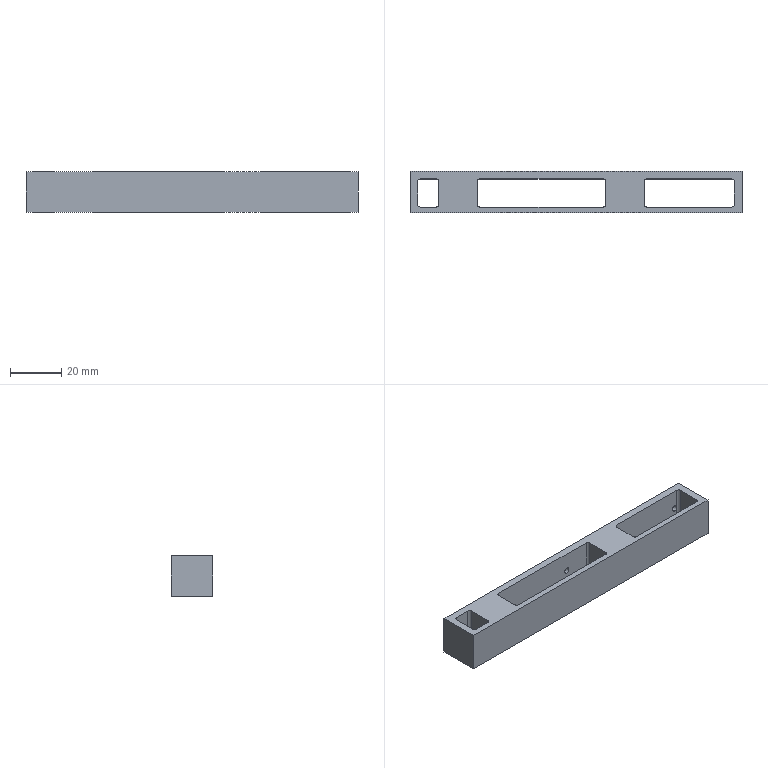NC program | NX | posted with a generic post | part box 130 x 16.2 x 16 mm
Lines 949 to 1955 of 19599:
(ZLEVEL_PROFILE_COPY_1_COPY , TOOL : D2)
N1872 T02 M6
N1874 G54
N1876 G17 G0 G90 X-57.176 Y-4.3 B0. C0. S9500 M3
N1878 G43 Z30. H2
N1880 Z0.401
N1882 G94 G1 Z-0.099 F1000.
N1884 X-56.888 Y-4.8
N1886 G3 X-56.715 Y-4.9 R0.2
N1888 G1 X-54.708 F2000.
N1890 Y-2.894
N1892 G3 X-54.808 Y-2.72 R0.2
N1894 G1 X-55.308 Y-2.432
N1896 Z0.401
N1898 G0 X-57.176 Y-4.3 Z0.301
N1900 G1 Z-0.199 F1000.
N1902 X-56.888 Y-4.8
N1904 G3 X-56.715 Y-4.9 R0.2
N1906 G1 X-54.708 F2000.
N1908 Y-2.894
N1910 G3 X-54.808 Y-2.72 R0.2
N1912 G1 X-55.308 Y-2.432
N1914 Z0.301
N1916 G0 X-57.176 Y-4.3 Z0.202
N1918 G1 Z-0.298 F1000.
N1920 X-56.888 Y-4.8
N1922 G3 X-56.715 Y-4.9 R0.2
N1924 G1 X-54.708 F2000.
N1926 Y-2.894
N1928 G3 X-54.808 Y-2.72 R0.2
N1930 G1 X-55.308 Y-2.432
N1932 Z0.202
N1934 G0 X-57.176 Y-4.3 Z0.102
N1936 G1 Z-0.398 F1000.
N1938 X-56.888 Y-4.8
N1940 G3 X-56.715 Y-4.9 R0.2
N1942 G1 X-54.708 F2000.
N1944 Y-2.894
N1946 G3 X-54.808 Y-2.72 R0.2
N1948 G1 X-55.308 Y-2.432
N1950 Z0.102
N1952 G0 X-57.176 Y-4.3 Z0.003
N1954 G1 Z-0.497 F1000.
N1956 X-56.888 Y-4.8
N1958 G3 X-56.715 Y-4.9 R0.2
N1960 G1 X-54.708 F2000.
N1962 Y-2.894
N1964 G3 X-54.808 Y-2.72 R0.2
N1966 G1 X-55.308 Y-2.432
N1968 Z0.003
N1970 G0 X-57.176 Y-4.3 Z-0.096
N1972 G1 Z-0.596 F1000.
N1974 X-56.888 Y-4.8
N1976 G3 X-56.715 Y-4.9 R0.2
N1978 G1 X-54.708 F2000.
N1980 Y-2.894
N1982 G3 X-54.808 Y-2.72 R0.2
N1984 G1 X-55.308 Y-2.432
N1986 Z-0.096
N1988 G0 X-57.176 Y-4.3 Z-0.196
N1990 G1 Z-0.696 F1000.
N1992 X-56.888 Y-4.8
N1994 G3 X-56.715 Y-4.9 R0.2
N1996 G1 X-54.708 F2000.
N1998 Y-2.894
N2000 G3 X-54.808 Y-2.72 R0.2
N2002 G1 X-55.308 Y-2.432
N2004 Z-0.196
N2006 G0 X-57.176 Y-4.3 Z-0.295
N2008 G1 Z-0.795 F1000.
N2010 X-56.888 Y-4.8
N2012 G3 X-56.715 Y-4.9 R0.2
N2014 G1 X-54.708 F2000.
N2016 Y-2.894
N2018 G3 X-54.808 Y-2.72 R0.2
N2020 G1 X-55.308 Y-2.432
N2022 Z-0.295
N2024 G0 X-57.176 Y-4.3 Z-0.394
N2026 G1 Z-0.894 F1000.
N2028 X-56.888 Y-4.8
N2030 G3 X-56.715 Y-4.9 R0.2
N2032 G1 X-54.708 F2000.
N2034 Y-2.894
N2036 G3 X-54.808 Y-2.72 R0.2
N2038 G1 X-55.308 Y-2.432
N2040 Z-0.394
N2042 G0 X-57.176 Y-4.3 Z-0.494
N2044 G1 Z-0.994 F1000.
N2046 X-56.888 Y-4.8
N2048 G3 X-56.715 Y-4.9 R0.2
N2050 G1 X-54.708 F2000.
N2052 Y-2.894
N2054 G3 X-54.808 Y-2.72 R0.2
N2056 G1 X-55.308 Y-2.432
N2058 Z-0.494
N2060 G0 X-57.176 Y-4.3 Z-0.593
N2062 G1 Z-1.093 F1000.
N2064 X-56.888 Y-4.8
N2066 G3 X-56.715 Y-4.9 R0.2
N2068 G1 X-54.708 F2000.
N2070 Y-2.894
N2072 G3 X-54.808 Y-2.72 R0.2
N2074 G1 X-55.308 Y-2.432
N2076 Z-0.593
N2078 G0 X-57.176 Y-4.3 Z-0.693
N2080 G1 Z-1.193 F1000.
N2082 X-56.888 Y-4.8
N2084 G3 X-56.715 Y-4.9 R0.2
N2086 G1 X-54.708 F2000.
N2088 Y-2.894
N2090 G3 X-54.808 Y-2.72 R0.2
N2092 G1 X-55.308 Y-2.432
N2094 Z-0.693
N2096 G0 X-57.176 Y-4.3 Z-0.792
N2098 G1 Z-1.292 F1000.
N2100 X-56.888 Y-4.8
N2102 G3 X-56.715 Y-4.9 R0.2
N2104 G1 X-54.708 F2000.
N2106 Y-2.894
N2108 G3 X-54.808 Y-2.72 R0.2
N2110 G1 X-55.308 Y-2.432
N2112 Z-0.792
N2114 G0 X-57.176 Y-4.3 Z-0.891
N2116 G1 Z-1.391 F1000.
N2118 X-56.888 Y-4.8
N2120 G3 X-56.715 Y-4.9 R0.2
N2122 G1 X-54.708 F2000.
N2124 Y-2.894
N2126 G3 X-54.808 Y-2.72 R0.2
N2128 G1 X-55.308 Y-2.432
N2130 Z-0.891
N2132 G0 X-57.176 Y-4.3 Z-0.991
N2134 G1 Z-1.491 F1000.
N2136 X-56.888 Y-4.8
N2138 G3 X-56.715 Y-4.9 R0.2
N2140 G1 X-54.708 F2000.
N2142 Y-2.894
N2144 G3 X-54.808 Y-2.72 R0.2
N2146 G1 X-55.308 Y-2.432
N2148 Z-0.991
N2150 G0 X-57.176 Y-4.3 Z-1.09
N2152 G1 Z-1.59 F1000.
N2154 X-56.888 Y-4.8
N2156 G3 X-56.715 Y-4.9 R0.2
N2158 G1 X-54.708 F2000.
N2160 Y-2.894
N2162 G3 X-54.808 Y-2.72 R0.2
N2164 G1 X-55.308 Y-2.432
N2166 Z-1.09
N2168 G0 X-57.176 Y-4.3 Z-1.189
N2170 G1 Z-1.689 F1000.
N2172 X-56.888 Y-4.8
N2174 G3 X-56.715 Y-4.9 R0.2
N2176 G1 X-54.708 F2000.
N2178 Y-2.894
N2180 G3 X-54.808 Y-2.72 R0.2
N2182 G1 X-55.308 Y-2.432
N2184 Z-1.189
N2186 G0 X-57.176 Y-4.3 Z-1.289
N2188 G1 Z-1.789 F1000.
N2190 X-56.888 Y-4.8
N2192 G3 X-56.715 Y-4.9 R0.2
N2194 G1 X-54.708 F2000.
N2196 Y-2.894
N2198 G3 X-54.808 Y-2.72 R0.2
N2200 G1 X-55.308 Y-2.432
N2202 Z-1.289
N2204 G0 X-57.176 Y-4.3 Z-1.388
N2206 G1 Z-1.888 F1000.
N2208 X-56.888 Y-4.8
N2210 G3 X-56.715 Y-4.9 R0.2
N2212 G1 X-54.708 F2000.
N2214 Y-2.894
N2216 G3 X-54.808 Y-2.72 R0.2
N2218 G1 X-55.308 Y-2.432
N2220 Z-1.388
N2222 G0 X-57.176 Y-4.3 Z-1.488
N2224 G1 Z-1.988 F1000.
N2226 X-56.888 Y-4.8
N2228 G3 X-56.715 Y-4.9 R0.2
N2230 G1 X-54.708 F2000.
N2232 Y-2.894
N2234 G3 X-54.808 Y-2.72 R0.2
N2236 G1 X-55.308 Y-2.432
N2238 Z-1.488
N2240 G0 X-57.176 Y-4.3 Z-1.587
N2242 G1 Z-2.087 F1000.
N2244 X-56.888 Y-4.8
N2246 G3 X-56.715 Y-4.9 R0.2
N2248 G1 X-54.708 F2000.
N2250 Y-2.894
N2252 G3 X-54.808 Y-2.72 R0.2
N2254 G1 X-55.308 Y-2.432
N2256 Z-1.587
N2258 G0 X-57.176 Y-4.3 Z-1.686
N2260 G1 Z-2.186 F1000.
N2262 X-56.888 Y-4.8
N2264 G3 X-56.715 Y-4.9 R0.2
N2266 G1 X-54.708 F2000.
N2268 Y-2.894
N2270 G3 X-54.808 Y-2.72 R0.2
N2272 G1 X-55.308 Y-2.432
N2274 Z-1.686
N2276 G0 X-57.176 Y-4.3 Z-1.786
N2278 G1 Z-2.286 F1000.
N2280 X-56.888 Y-4.8
N2282 G3 X-56.715 Y-4.9 R0.2
N2284 G1 X-54.708 F2000.
N2286 Y-2.894
N2288 G3 X-54.808 Y-2.72 R0.2
N2290 G1 X-55.308 Y-2.432
N2292 Z-1.786
N2294 G0 X-57.176 Y-4.3 Z-1.885
N2296 G1 Z-2.385 F1000.
N2298 X-56.888 Y-4.8
N2300 G3 X-56.715 Y-4.9 R0.2
N2302 G1 X-54.708 F2000.
N2304 Y-2.894
N2306 G3 X-54.808 Y-2.72 R0.2
N2308 G1 X-55.308 Y-2.432
N2310 Z-1.885
N2312 G0 X-57.176 Y-4.3 Z-1.984
N2314 G1 Z-2.484 F1000.
N2316 X-56.888 Y-4.8
N2318 G3 X-56.715 Y-4.9 R0.2
N2320 G1 X-54.708 F2000.
N2322 Y-2.894
N2324 G3 X-54.808 Y-2.72 R0.2
N2326 G1 X-55.308 Y-2.432
N2328 Z-1.984
N2330 G0 X-57.176 Y-4.3 Z-2.084
N2332 G1 Z-2.584 F1000.
N2334 X-56.888 Y-4.8
N2336 G3 X-56.715 Y-4.9 R0.2
N2338 G1 X-54.708 F2000.
N2340 Y-2.894
N2342 G3 X-54.808 Y-2.72 R0.2
N2344 G1 X-55.308 Y-2.432
N2346 Z-2.084
N2348 G0 X-57.176 Y-4.3 Z-2.183
N2350 G1 Z-2.683 F1000.
N2352 X-56.888 Y-4.8
N2354 G3 X-56.715 Y-4.9 R0.2
N2356 G1 X-54.708 F2000.
N2358 Y-2.894
N2360 G3 X-54.808 Y-2.72 R0.2
N2362 G1 X-55.308 Y-2.432
N2364 Z-2.183
N2366 G0 X-57.176 Y-4.3 Z-2.283
N2368 G1 Z-2.783 F1000.
N2370 X-56.888 Y-4.8
N2372 G3 X-56.715 Y-4.9 R0.2
N2374 G1 X-54.708 F2000.
N2376 Y-2.894
N2378 G3 X-54.808 Y-2.72 R0.2
N2380 G1 X-55.308 Y-2.432
N2382 Z-2.283
N2384 G0 X-57.176 Y-4.3 Z-2.382
N2386 G1 Z-2.882 F1000.
N2388 X-56.888 Y-4.8
N2390 G3 X-56.715 Y-4.9 R0.2
N2392 G1 X-54.708 F2000.
N2394 Y-2.894
N2396 G3 X-54.808 Y-2.72 R0.2
N2398 G1 X-55.308 Y-2.432
N2400 Z-2.382
N2402 G0 X-57.176 Y-4.3 Z-2.481
N2404 G1 Z-2.981 F1000.
N2406 X-56.888 Y-4.8
N2408 G3 X-56.715 Y-4.9 R0.2
N2410 G1 X-54.708 F2000.
N2412 Y-2.894
N2414 G3 X-54.808 Y-2.72 R0.2
N2416 G1 X-55.308 Y-2.432
N2418 Z-2.481
N2420 G0 X-57.176 Y-4.3 Z-2.581
N2422 G1 Z-3.081 F1000.
N2424 X-56.888 Y-4.8
N2426 G3 X-56.715 Y-4.9 R0.2
N2428 G1 X-54.708 F2000.
N2430 Y-2.894
N2432 G3 X-54.808 Y-2.72 R0.2
N2434 G1 X-55.308 Y-2.432
N2436 Z-2.581
N2438 G0 X-57.176 Y-4.3 Z-2.68
N2440 G1 Z-3.18 F1000.
N2442 X-56.888 Y-4.8
N2444 G3 X-56.715 Y-4.9 R0.2
N2446 G1 X-54.708 F2000.
N2448 Y-2.894
N2450 G3 X-54.808 Y-2.72 R0.2
N2452 G1 X-55.308 Y-2.432
N2454 Z-2.68
N2456 G0 X-57.176 Y-4.3 Z-2.78
N2458 G1 Z-3.28 F1000.
N2460 X-56.888 Y-4.8
N2462 G3 X-56.715 Y-4.9 R0.2
N2464 G1 X-54.708 F2000.
N2466 Y-2.894
N2468 G3 X-54.808 Y-2.72 R0.2
N2470 G1 X-55.308 Y-2.432
N2472 Z-2.78
N2474 G0 X-57.176 Y-4.3 Z-2.879
N2476 G1 Z-3.379 F1000.
N2478 X-56.888 Y-4.8
N2480 G3 X-56.715 Y-4.9 R0.2
N2482 G1 X-54.708 F2000.
N2484 Y-2.894
N2486 G3 X-54.808 Y-2.72 R0.2
N2488 G1 X-55.308 Y-2.432
N2490 Z-2.879
N2492 G0 X-57.176 Y-4.3 Z-2.978
N2494 G1 Z-3.478 F1000.
N2496 X-56.888 Y-4.8
N2498 G3 X-56.715 Y-4.9 R0.2
N2500 G1 X-54.708 F2000.
N2502 Y-2.894
N2504 G3 X-54.808 Y-2.72 R0.2
N2506 G1 X-55.308 Y-2.432
N2508 Z-2.978
N2510 G0 X-57.176 Y-4.3 Z-3.078
N2512 G1 Z-3.578 F1000.
N2514 X-56.888 Y-4.8
N2516 G3 X-56.715 Y-4.9 R0.2
N2518 G1 X-54.708 F2000.
N2520 Y-2.894
N2522 G3 X-54.808 Y-2.72 R0.2
N2524 G1 X-55.308 Y-2.432
N2526 Z-3.078
N2528 G0 X-57.176 Y-4.3 Z-3.177
N2530 G1 Z-3.677 F1000.
N2532 X-56.888 Y-4.8
N2534 G3 X-56.715 Y-4.9 R0.2
N2536 G1 X-54.708 F2000.
N2538 Y-2.894
N2540 G3 X-54.808 Y-2.72 R0.2
N2542 G1 X-55.308 Y-2.432
N2544 Z-3.177
N2546 G0 X-57.176 Y-4.3 Z-3.276
N2548 G1 Z-3.776 F1000.
N2550 X-56.888 Y-4.8
N2552 G3 X-56.715 Y-4.9 R0.2
N2554 G1 X-54.708 F2000.
N2556 Y-2.894
N2558 G3 X-54.808 Y-2.72 R0.2
N2560 G1 X-55.308 Y-2.432
N2562 Z-3.276
N2564 G0 X-57.176 Y-4.3 Z-3.376
N2566 G1 Z-3.876 F1000.
N2568 X-56.888 Y-4.8
N2570 G3 X-56.715 Y-4.9 R0.2
N2572 G1 X-54.708 F2000.
N2574 Y-2.894
N2576 G3 X-54.808 Y-2.72 R0.2
N2578 G1 X-55.308 Y-2.432
N2580 Z-3.376
N2582 G0 X-57.176 Y-4.3 Z-3.475
N2584 G1 Z-3.975 F1000.
N2586 X-56.888 Y-4.8
N2588 G3 X-56.715 Y-4.9 R0.2
N2590 G1 X-54.708 F2000.
N2592 Y-2.894
N2594 G3 X-54.808 Y-2.72 R0.2
N2596 G1 X-55.308 Y-2.432
N2598 Z-3.475
N2600 G0 X-57.176 Y-4.3 Z-3.575
N2602 G1 Z-4.075 F1000.
N2604 X-56.888 Y-4.8
N2606 G3 X-56.715 Y-4.9 R0.2
N2608 G1 X-54.708 F2000.
N2610 Y-2.894
N2612 G3 X-54.808 Y-2.72 R0.2
N2614 G1 X-55.308 Y-2.432
N2616 Z-3.575
N2618 G0 X-57.176 Y-4.3 Z-3.674
N2620 G1 Z-4.174 F1000.
N2622 X-56.888 Y-4.8
N2624 G3 X-56.715 Y-4.9 R0.2
N2626 G1 X-54.708 F2000.
N2628 Y-2.894
N2630 G3 X-54.808 Y-2.72 R0.2
N2632 G1 X-55.308 Y-2.432
N2634 Z-3.674
N2636 G0 X-57.176 Y-4.3 Z-3.773
N2638 G1 Z-4.273 F1000.
N2640 X-56.888 Y-4.8
N2642 G3 X-56.715 Y-4.9 R0.2
N2644 G1 X-54.708 F2000.
N2646 Y-2.894
N2648 G3 X-54.808 Y-2.72 R0.2
N2650 G1 X-55.308 Y-2.432
N2652 Z-3.773
N2654 G0 X-57.176 Y-4.3 Z-3.873
N2656 G1 Z-4.373 F1000.
N2658 X-56.888 Y-4.8
N2660 G3 X-56.715 Y-4.9 R0.2
N2662 G1 X-54.708 F2000.
N2664 Y-2.894
N2666 G3 X-54.808 Y-2.72 R0.2
N2668 G1 X-55.308 Y-2.432
N2670 Z-3.873
N2672 G0 X-57.176 Y-4.3 Z-3.972
N2674 G1 Z-4.472 F1000.
N2676 X-56.888 Y-4.8
N2678 G3 X-56.715 Y-4.9 R0.2
N2680 G1 X-54.708 F2000.
N2682 Y-2.894
N2684 G3 X-54.808 Y-2.72 R0.2
N2686 G1 X-55.308 Y-2.432
N2688 Z-3.972
N2690 G0 X-57.176 Y-4.3 Z-4.071
N2692 G1 Z-4.571 F1000.
N2694 X-56.888 Y-4.8
N2696 G3 X-56.715 Y-4.9 R0.2
N2698 G1 X-54.708 F2000.
N2700 Y-2.894
N2702 G3 X-54.808 Y-2.72 R0.2
N2704 G1 X-55.308 Y-2.432
N2706 Z-4.071
N2708 G0 X-57.176 Y-4.3 Z-4.171
N2710 G1 Z-4.671 F1000.
N2712 X-56.888 Y-4.8
N2714 G3 X-56.715 Y-4.9 R0.2
N2716 G1 X-54.708 F2000.
N2718 Y-2.894
N2720 G3 X-54.808 Y-2.72 R0.2
N2722 G1 X-55.308 Y-2.432
N2724 Z-4.171
N2726 G0 X-57.176 Y-4.3 Z-4.27
N2728 G1 Z-4.77 F1000.
N2730 X-56.888 Y-4.8
N2732 G3 X-56.715 Y-4.9 R0.2
N2734 G1 X-54.708 F2000.
N2736 Y-2.894
N2738 G3 X-54.808 Y-2.72 R0.2
N2740 G1 X-55.308 Y-2.432
N2742 Z-4.27
N2744 G0 X-57.176 Y-4.3 Z-4.37
N2746 G1 Z-4.87 F1000.
N2748 X-56.888 Y-4.8
N2750 G3 X-56.715 Y-4.9 R0.2
N2752 G1 X-54.708 F2000.
N2754 Y-2.894
N2756 G3 X-54.808 Y-2.72 R0.2
N2758 G1 X-55.308 Y-2.432
N2760 Z-4.37
N2762 G0 X-57.176 Y-4.3 Z-4.469
N2764 G1 Z-4.969 F1000.
N2766 X-56.888 Y-4.8
N2768 G3 X-56.715 Y-4.9 R0.2
N2770 G1 X-54.708 F2000.
N2772 Y-2.894
N2774 G3 X-54.808 Y-2.72 R0.2
N2776 G1 X-55.308 Y-2.432
N2778 Z-4.469
N2780 G0 X-57.176 Y-4.3 Z-4.568
N2782 G1 Z-5.068 F1000.
N2784 X-56.888 Y-4.8
N2786 G3 X-56.715 Y-4.9 R0.2
N2788 G1 X-54.708 F2000.
N2790 Y-2.894
N2792 G3 X-54.808 Y-2.72 R0.2
N2794 G1 X-55.308 Y-2.432
N2796 Z-4.568
N2798 G0 X-57.176 Y-4.3 Z-4.668
N2800 G1 Z-5.168 F1000.
N2802 X-56.888 Y-4.8
N2804 G3 X-56.715 Y-4.9 R0.2
N2806 G1 X-54.708 F2000.
N2808 Y-2.894
N2810 G3 X-54.808 Y-2.72 R0.2
N2812 G1 X-55.308 Y-2.432
N2814 Z-4.668
N2816 G0 X-57.176 Y-4.3 Z-4.767
N2818 G1 Z-5.267 F1000.
N2820 X-56.888 Y-4.8
N2822 G3 X-56.715 Y-4.9 R0.2
N2824 G1 X-54.708 F2000.
N2826 Y-2.894
N2828 G3 X-54.808 Y-2.72 R0.2
N2830 G1 X-55.308 Y-2.432
N2832 Z-4.767
N2834 G0 X-57.176 Y-4.3 Z-4.866
N2836 G1 Z-5.366 F1000.
N2838 X-56.888 Y-4.8
N2840 G3 X-56.715 Y-4.9 R0.2
N2842 G1 X-54.708 F2000.
N2844 Y-2.894
N2846 G3 X-54.808 Y-2.72 R0.2
N2848 G1 X-55.308 Y-2.432
N2850 Z-4.866
N2852 G0 X-57.176 Y-4.3 Z-4.966
N2854 G1 Z-5.466 F1000.
N2856 X-56.888 Y-4.8
N2858 G3 X-56.715 Y-4.9 R0.2
N2860 G1 X-54.708 F2000.
N2862 Y-2.894
N2864 G3 X-54.808 Y-2.72 R0.2
N2866 G1 X-55.308 Y-2.432
N2868 Z-4.966
N2870 G0 X-57.176 Y-4.3 Z-5.065
N2872 G1 Z-5.565 F1000.
N2874 X-56.888 Y-4.8
N2876 G3 X-56.715 Y-4.9 R0.2
N2878 G1 X-54.708 F2000.
N2880 Y-2.894
N2882 G3 X-54.808 Y-2.72 R0.2
N2884 G1 X-55.308 Y-2.432
N2886 Z-5.065
N2888 G0 X-57.176 Y-4.3 Z-5.165
N2890 G1 Z-5.665 F1000.
N2892 X-56.888 Y-4.8
N2894 G3 X-56.715 Y-4.9 R0.2
N2896 G1 X-54.708 F2000.
N2898 Y-2.894
N2900 G3 X-54.808 Y-2.72 R0.2
N2902 G1 X-55.308 Y-2.432
N2904 Z-5.165
N2906 G0 X-57.176 Y-4.3 Z-5.264
N2908 G1 Z-5.764 F1000.
N2910 X-56.888 Y-4.8
N2912 G3 X-56.715 Y-4.9 R0.2
N2914 G1 X-54.708 F2000.
N2916 Y-2.894
N2918 G3 X-54.808 Y-2.72 R0.2
N2920 G1 X-55.308 Y-2.432
N2922 Z-5.264
N2924 G0 X-57.176 Y-4.3 Z-5.363
N2926 G1 Z-5.863 F1000.
N2928 X-56.888 Y-4.8
N2930 G3 X-56.715 Y-4.9 R0.2
N2932 G1 X-54.708 F2000.
N2934 Y-2.894
N2936 G3 X-54.808 Y-2.72 R0.2
N2938 G1 X-55.308 Y-2.432
N2940 Z-5.363
N2942 G0 X-57.176 Y-4.3 Z-5.463
N2944 G1 Z-5.963 F1000.
N2946 X-56.888 Y-4.8
N2948 G3 X-56.715 Y-4.9 R0.2
N2950 G1 X-54.708 F2000.
N2952 Y-2.894
N2954 G3 X-54.808 Y-2.72 R0.2
N2956 G1 X-55.308 Y-2.432
N2958 Z-5.463
N2960 G0 X-57.176 Y-4.3 Z-5.562
N2962 G1 Z-6.062 F1000.
N2964 X-56.888 Y-4.8
N2966 G3 X-56.715 Y-4.9 R0.2
N2968 G1 X-54.708 F2000.
N2970 Y-2.894
N2972 G3 X-54.808 Y-2.72 R0.2
N2974 G1 X-55.308 Y-2.432
N2976 Z-5.562
N2978 G0 X-57.176 Y-4.3 Z-5.661
N2980 G1 Z-6.161 F1000.
N2982 X-56.888 Y-4.8
N2984 G3 X-56.715 Y-4.9 R0.2
N2986 G1 X-54.708 F2000.
N2988 Y-2.894
N2990 G3 X-54.808 Y-2.72 R0.2
N2992 G1 X-55.308 Y-2.432
N2994 Z-5.661
N2996 G0 X-57.176 Y-4.3 Z-5.761
N2998 G1 Z-6.261 F1000.
N3000 X-56.888 Y-4.8
N3002 G3 X-56.715 Y-4.9 R0.2
N3004 G1 X-54.708 F2000.
N3006 Y-2.894
N3008 G3 X-54.808 Y-2.72 R0.2
N3010 G1 X-55.308 Y-2.432
N3012 Z-5.761
N3014 G0 X-57.176 Y-4.3 Z-5.86
N3016 G1 Z-6.36 F1000.
N3018 X-56.888 Y-4.8
N3020 G3 X-56.715 Y-4.9 R0.2
N3022 G1 X-54.708 F2000.
N3024 Y-2.894
N3026 G3 X-54.808 Y-2.72 R0.2
N3028 G1 X-55.308 Y-2.432
N3030 Z-5.86
N3032 G0 X-57.176 Y-4.3 Z-5.96
N3034 G1 Z-6.46 F1000.
N3036 X-56.888 Y-4.8
N3038 G3 X-56.715 Y-4.9 R0.2
N3040 G1 X-54.708 F2000.
N3042 Y-2.894
N3044 G3 X-54.808 Y-2.72 R0.2
N3046 G1 X-55.308 Y-2.432
N3048 Z-5.96
N3050 G0 X-57.176 Y-4.3 Z-6.059
N3052 G1 Z-6.559 F1000.
N3054 X-56.888 Y-4.8
N3056 G3 X-56.715 Y-4.9 R0.2
N3058 G1 X-54.708 F2000.
N3060 Y-2.894
N3062 G3 X-54.808 Y-2.72 R0.2
N3064 G1 X-55.308 Y-2.432
N3066 Z-6.059
N3068 G0 X-57.176 Y-4.3 Z-6.158
N3070 G1 Z-6.658 F1000.
N3072 X-56.888 Y-4.8
N3074 G3 X-56.715 Y-4.9 R0.2
N3076 G1 X-54.708 F2000.
N3078 Y-2.894
N3080 G3 X-54.808 Y-2.72 R0.2
N3082 G1 X-55.308 Y-2.432
N3084 Z-6.158
N3086 G0 X-57.176 Y-4.3 Z-6.258
N3088 G1 Z-6.758 F1000.
N3090 X-56.888 Y-4.8
N3092 G3 X-56.715 Y-4.9 R0.2
N3094 G1 X-54.708 F2000.
N3096 Y-2.894
N3098 G3 X-54.808 Y-2.72 R0.2
N3100 G1 X-55.308 Y-2.432
N3102 Z-6.258
N3104 G0 X-57.176 Y-4.3 Z-6.357
N3106 G1 Z-6.857 F1000.
N3108 X-56.888 Y-4.8
N3110 G3 X-56.715 Y-4.9 R0.2
N3112 G1 X-54.708 F2000.
N3114 Y-2.894
N3116 G3 X-54.808 Y-2.72 R0.2
N3118 G1 X-55.308 Y-2.432
N3120 Z-6.357
N3122 G0 X-57.176 Y-4.3 Z-6.457
N3124 G1 Z-6.957 F1000.
N3126 X-56.888 Y-4.8
N3128 G3 X-56.715 Y-4.9 R0.2
N3130 G1 X-54.708 F2000.
N3132 Y-2.894
N3134 G3 X-54.808 Y-2.72 R0.2
N3136 G1 X-55.308 Y-2.432
N3138 Z-6.457
N3140 G0 X-57.176 Y-4.3 Z-6.556
N3142 G1 Z-7.056 F1000.
N3144 X-56.888 Y-4.8
N3146 G3 X-56.715 Y-4.9 R0.2
N3148 G1 X-54.708 F2000.
N3150 Y-2.894
N3152 G3 X-54.808 Y-2.72 R0.2
N3154 G1 X-55.308 Y-2.432
N3156 Z-6.556
N3158 G0 X-57.176 Y-4.3 Z-6.655
N3160 G1 Z-7.155 F1000.
N3162 X-56.888 Y-4.8
N3164 G3 X-56.715 Y-4.9 R0.2
N3166 G1 X-54.708 F2000.
N3168 Y-2.894
N3170 G3 X-54.808 Y-2.72 R0.2
N3172 G1 X-55.308 Y-2.432
N3174 Z-6.655
N3176 G0 X-57.176 Y-4.3 Z-6.755
N3178 G1 Z-7.255 F1000.
N3180 X-56.888 Y-4.8
N3182 G3 X-56.715 Y-4.9 R0.2
N3184 G1 X-54.708 F2000.
N3186 Y-2.894
N3188 G3 X-54.808 Y-2.72 R0.2
N3190 G1 X-55.308 Y-2.432
N3192 Z-6.755
N3194 G0 X-57.176 Y-4.3 Z-6.854
N3196 G1 Z-7.354 F1000.
N3198 X-56.888 Y-4.8
N3200 G3 X-56.715 Y-4.9 R0.2
N3202 G1 X-54.708 F2000.
N3204 Y-2.894
N3206 G3 X-54.808 Y-2.72 R0.2
N3208 G1 X-55.308 Y-2.432
N3210 Z-6.854
N3212 G0 X-57.176 Y-4.3 Z-6.953
N3214 G1 Z-7.453 F1000.
N3216 X-56.888 Y-4.8
N3218 G3 X-56.715 Y-4.9 R0.2
N3220 G1 X-54.708 F2000.
N3222 Y-2.894
N3224 G3 X-54.808 Y-2.72 R0.2
N3226 G1 X-55.308 Y-2.432
N3228 Z-6.953
N3230 G0 X-57.176 Y-4.3 Z-7.053
N3232 G1 Z-7.553 F1000.
N3234 X-56.888 Y-4.8
N3236 G3 X-56.715 Y-4.9 R0.2
N3238 G1 X-54.708 F2000.
N3240 Y-2.894
N3242 G3 X-54.808 Y-2.72 R0.2
N3244 G1 X-55.308 Y-2.432
N3246 Z-7.053
N3248 G0 X-57.176 Y-4.3 Z-7.152
N3250 G1 Z-7.652 F1000.
N3252 X-56.888 Y-4.8
N3254 G3 X-56.715 Y-4.9 R0.2
N3256 G1 X-54.708 F2000.
N3258 Y-2.894
N3260 G3 X-54.808 Y-2.72 R0.2
N3262 G1 X-55.308 Y-2.432
N3264 Z-7.152
N3266 G0 X-57.176 Y-4.3 Z-7.252
N3268 G1 Z-7.752 F1000.
N3270 X-56.888 Y-4.8
N3272 G3 X-56.715 Y-4.9 R0.2
N3274 G1 X-54.708 F2000.
N3276 Y-2.894
N3278 G3 X-54.808 Y-2.72 R0.2
N3280 G1 X-55.308 Y-2.432
N3282 Z-7.252
N3284 G0 X-57.176 Y-4.3 Z-7.351
N3286 G1 Z-7.851 F1000.
N3288 X-56.888 Y-4.8
N3290 G3 X-56.715 Y-4.9 R0.2
N3292 G1 X-54.708 F2000.
N3294 Y-2.894
N3296 G3 X-54.808 Y-2.72 R0.2
N3298 G1 X-55.308 Y-2.432
N3300 Z-7.351
N3302 G0 X-57.176 Y-4.3 Z-7.45
N3304 G1 Z-7.95 F1000.
N3306 X-56.888 Y-4.8
N3308 G3 X-56.715 Y-4.9 R0.2
N3310 G1 X-54.708 F2000.
N3312 Y-2.894
N3314 G3 X-54.808 Y-2.72 R0.2
N3316 G1 X-55.308 Y-2.432
N3318 Z-7.45
N3320 G0 X-57.176 Y-4.3 Z-7.55
N3322 G1 Z-8.05 F1000.
N3324 X-56.888 Y-4.8
N3326 G3 X-56.715 Y-4.9 R0.2
N3328 G1 X-54.708 F2000.
N3330 Y-2.894
N3332 G3 X-54.808 Y-2.72 R0.2
N3334 G1 X-55.308 Y-2.432
N3336 Z-7.55
N3338 G0 X-57.176 Y-4.3 Z-7.649
N3340 G1 Z-8.149 F1000.
N3342 X-56.888 Y-4.8
N3344 G3 X-56.715 Y-4.9 R0.2
N3346 G1 X-54.708 F2000.
N3348 Y-2.894
N3350 G3 X-54.808 Y-2.72 R0.2
N3352 G1 X-55.308 Y-2.432
N3354 Z-7.649
N3356 G0 X-57.176 Y-4.3 Z-7.748
N3358 G1 Z-8.248 F1000.
N3360 X-56.888 Y-4.8
N3362 G3 X-56.715 Y-4.9 R0.2
N3364 G1 X-54.708 F2000.
N3366 Y-2.894
N3368 G3 X-54.808 Y-2.72 R0.2
N3370 G1 X-55.308 Y-2.432
N3372 Z-7.748
N3374 G0 X-57.176 Y-4.3 Z-7.848
N3376 G1 Z-8.348 F1000.
N3378 X-56.888 Y-4.8
N3380 G3 X-56.715 Y-4.9 R0.2
N3382 G1 X-54.708 F2000.
N3384 Y-2.894
N3386 G3 X-54.808 Y-2.72 R0.2
N3388 G1 X-55.308 Y-2.432
N3390 Z-7.848
N3392 G0 X-57.176 Y-4.3 Z-7.947
N3394 G1 Z-8.447 F1000.
N3396 X-56.888 Y-4.8
N3398 G3 X-56.715 Y-4.9 R0.2
N3400 G1 X-54.708 F2000.
N3402 Y-2.894
N3404 G3 X-54.808 Y-2.72 R0.2
N3406 G1 X-55.308 Y-2.432
N3408 Z-7.947
N3410 G0 X-57.176 Y-4.3 Z-8.047
N3412 G1 Z-8.547 F1000.
N3414 X-56.888 Y-4.8
N3416 G3 X-56.715 Y-4.9 R0.2
N3418 G1 X-54.708 F2000.
N3420 Y-2.894
N3422 G3 X-54.808 Y-2.72 R0.2
N3424 G1 X-55.308 Y-2.432
N3426 Z-8.047
N3428 G0 X-57.176 Y-4.3 Z-8.146
N3430 G1 Z-8.646 F1000.
N3432 X-56.888 Y-4.8
N3434 G3 X-56.715 Y-4.9 R0.2
N3436 G1 X-54.708 F2000.
N3438 Y-2.894
N3440 G3 X-54.808 Y-2.72 R0.2
N3442 G1 X-55.308 Y-2.432
N3444 Z-8.146
N3446 G0 X-57.176 Y-4.3 Z-8.245
N3448 G1 Z-8.745 F1000.
N3450 X-56.888 Y-4.8
N3452 G3 X-56.715 Y-4.9 R0.2
N3454 G1 X-54.708 F2000.
N3456 Y-2.894
N3458 G3 X-54.808 Y-2.72 R0.2
N3460 G1 X-55.308 Y-2.432
N3462 Z-8.245
N3464 G0 X-57.176 Y-4.3 Z-8.345
N3466 G1 Z-8.845 F1000.
N3468 X-56.888 Y-4.8
N3470 G3 X-56.715 Y-4.9 R0.2
N3472 G1 X-54.708 F2000.
N3474 Y-2.894
N3476 G3 X-54.808 Y-2.72 R0.2
N3478 G1 X-55.308 Y-2.432
N3480 Z-8.345
N3482 G0 X-57.176 Y-4.3 Z-8.444
N3484 G1 Z-8.944 F1000.
N3486 X-56.888 Y-4.8
N3488 G3 X-56.715 Y-4.9 R0.2
N3490 G1 X-54.708 F2000.
N3492 Y-2.894
N3494 G3 X-54.808 Y-2.72 R0.2
N3496 G1 X-55.308 Y-2.432
N3498 Z-8.444
N3500 G0 X-57.176 Y-4.3 Z-8.543
N3502 G1 Z-9.043 F1000.
N3504 X-56.888 Y-4.8
N3506 G3 X-56.715 Y-4.9 R0.2
N3508 G1 X-54.708 F2000.
N3510 Y-2.894
N3512 G3 X-54.808 Y-2.72 R0.2
N3514 G1 X-55.308 Y-2.432
N3516 Z-8.543
N3518 G0 X-57.176 Y-4.3 Z-8.643
N3520 G1 Z-9.143 F1000.
N3522 X-56.888 Y-4.8
N3524 G3 X-56.715 Y-4.9 R0.2
N3526 G1 X-54.708 F2000.
N3528 Y-2.894
N3530 G3 X-54.808 Y-2.72 R0.2
N3532 G1 X-55.308 Y-2.432
N3534 Z-8.643
N3536 G0 X-57.176 Y-4.3 Z-8.742
N3538 G1 Z-9.242 F1000.
N3540 X-56.888 Y-4.8
N3542 G3 X-56.715 Y-4.9 R0.2
N3544 G1 X-54.708 F2000.
N3546 Y-2.894
N3548 G3 X-54.808 Y-2.72 R0.2
N3550 G1 X-55.308 Y-2.432
N3552 Z-8.742
N3554 G0 X-57.176 Y-4.3 Z-8.842
N3556 G1 Z-9.342 F1000.
N3558 X-56.888 Y-4.8
N3560 G3 X-56.715 Y-4.9 R0.2
N3562 G1 X-54.708 F2000.
N3564 Y-2.894
N3566 G3 X-54.808 Y-2.72 R0.2
N3568 G1 X-55.308 Y-2.432
N3570 Z-8.842
N3572 G0 X-57.176 Y-4.3 Z-8.941
N3574 G1 Z-9.441 F1000.
N3576 X-56.888 Y-4.8
N3578 G3 X-56.715 Y-4.9 R0.2
N3580 G1 X-54.708 F2000.
N3582 Y-2.894
N3584 G3 X-54.808 Y-2.72 R0.2
N3586 G1 X-55.308 Y-2.432
N3588 Z-8.941
N3590 G0 X-57.176 Y-4.3 Z-9.04
N3592 G1 Z-9.54 F1000.
N3594 X-56.888 Y-4.8
N3596 G3 X-56.715 Y-4.9 R0.2
N3598 G1 X-54.708 F2000.
N3600 Y-2.894
N3602 G3 X-54.808 Y-2.72 R0.2
N3604 G1 X-55.308 Y-2.432
N3606 Z-9.04
N3608 G0 X-57.176 Y-4.3 Z-9.14
N3610 G1 Z-9.64 F1000.
N3612 X-56.888 Y-4.8
N3614 G3 X-56.715 Y-4.9 R0.2
N3616 G1 X-54.708 F2000.
N3618 Y-2.894
N3620 G3 X-54.808 Y-2.72 R0.2
N3622 G1 X-55.308 Y-2.432
N3624 Z-9.14
N3626 G0 X-57.176 Y-4.3 Z-9.239
N3628 G1 Z-9.739 F1000.
N3630 X-56.888 Y-4.8
N3632 G3 X-56.715 Y-4.9 R0.2
N3634 G1 X-54.708 F2000.
N3636 Y-2.894
N3638 G3 X-54.808 Y-2.72 R0.2
N3640 G1 X-55.308 Y-2.432
N3642 Z-9.239
N3644 G0 X-57.176 Y-4.3 Z-9.339
N3646 G1 Z-9.839 F1000.
N3648 X-56.888 Y-4.8
N3650 G3 X-56.715 Y-4.9 R0.2
N3652 G1 X-54.708 F2000.
N3654 Y-2.894
N3656 G3 X-54.808 Y-2.72 R0.2
N3658 G1 X-55.308 Y-2.432
N3660 Z-9.339
N3662 G0 X-57.176 Y-4.3 Z-9.438
N3664 G1 Z-9.938 F1000.
N3666 X-56.888 Y-4.8
N3668 G3 X-56.715 Y-4.9 R0.2
N3670 G1 X-54.708 F2000.
N3672 Y-2.894
N3674 G3 X-54.808 Y-2.72 R0.2
N3676 G1 X-55.308 Y-2.432
N3678 Z-9.438
N3680 G0 X-57.176 Y-4.3 Z-9.537
N3682 G1 Z-10.037 F1000.
N3684 X-56.888 Y-4.8
N3686 G3 X-56.715 Y-4.9 R0.2
N3688 G1 X-54.708 F2000.
N3690 Y-2.894
N3692 G3 X-54.808 Y-2.72 R0.2
N3694 G1 X-55.308 Y-2.432
N3696 Z-9.537
N3698 G0 X-57.176 Y-4.3 Z-9.637
N3700 G1 Z-10.137 F1000.
N3702 X-56.888 Y-4.8
N3704 G3 X-56.715 Y-4.9 R0.2
N3706 G1 X-54.708 F2000.
N3708 Y-2.894
N3710 G3 X-54.808 Y-2.72 R0.2
N3712 G1 X-55.308 Y-2.432
N3714 Z-9.637
N3716 G0 X-57.176 Y-4.3 Z-9.736
N3718 G1 Z-10.236 F1000.
N3720 X-56.888 Y-4.8
N3722 G3 X-56.715 Y-4.9 R0.2
N3724 G1 X-54.708 F2000.
N3726 Y-2.894
N3728 G3 X-54.808 Y-2.72 R0.2
N3730 G1 X-55.308 Y-2.432
N3732 Z-9.736
N3734 G0 X-57.176 Y-4.3 Z-9.835
N3736 G1 Z-10.335 F1000.
N3738 X-56.888 Y-4.8
N3740 G3 X-56.715 Y-4.9 R0.2
N3742 G1 X-54.708 F2000.
N3744 Y-2.894
N3746 G3 X-54.808 Y-2.72 R0.2
N3748 G1 X-55.308 Y-2.432
N3750 Z-9.835
N3752 G0 X-57.176 Y-4.3 Z-9.935
N3754 G1 Z-10.435 F1000.
N3756 X-56.888 Y-4.8
N3758 G3 X-56.715 Y-4.9 R0.2
N3760 G1 X-54.708 F2000.
N3762 Y-2.894
N3764 G3 X-54.808 Y-2.72 R0.2
N3766 G1 X-55.308 Y-2.432
N3768 Z-9.935
N3770 G0 X-57.176 Y-4.3 Z-10.034
N3772 G1 Z-10.534 F1000.
N3774 X-56.888 Y-4.8
N3776 G3 X-56.715 Y-4.9 R0.2
N3778 G1 X-54.708 F2000.
N3780 Y-2.894
N3782 G3 X-54.808 Y-2.72 R0.2
N3784 G1 X-55.308 Y-2.432
N3786 Z-10.034
N3788 G0 X-57.176 Y-4.3 Z-10.134
N3790 G1 Z-10.634 F1000.
N3792 X-56.888 Y-4.8
N3794 G3 X-56.715 Y-4.9 R0.2
N3796 G1 X-54.708 F2000.
N3798 Y-2.894
N3800 G3 X-54.808 Y-2.72 R0.2
N3802 G1 X-55.308 Y-2.432
N3804 Z-10.134
N3806 G0 X-57.176 Y-4.3 Z-10.233
N3808 G1 Z-10.733 F1000.
N3810 X-56.888 Y-4.8
N3812 G3 X-56.715 Y-4.9 R0.2
N3814 G1 X-54.708 F2000.
N3816 Y-2.894
N3818 G3 X-54.808 Y-2.72 R0.2
N3820 G1 X-55.308 Y-2.432
N3822 Z-10.233
N3824 G0 X-57.176 Y-4.3 Z-10.332
N3826 G1 Z-10.832 F1000.
N3828 X-56.888 Y-4.8
N3830 G3 X-56.715 Y-4.9 R0.2
N3832 G1 X-54.708 F2000.
N3834 Y-2.894
N3836 G3 X-54.808 Y-2.72 R0.2
N3838 G1 X-55.308 Y-2.432
N3840 Z-10.332
N3842 G0 X-57.176 Y-4.3 Z-10.432
N3844 G1 Z-10.932 F1000.
N3846 X-56.888 Y-4.8
N3848 G3 X-56.715 Y-4.9 R0.2
N3850 G1 X-54.708 F2000.
N3852 Y-2.894
N3854 G3 X-54.808 Y-2.72 R0.2
N3856 G1 X-55.308 Y-2.432
N3858 Z-10.432
N3860 G0 X-57.176 Y-4.3 Z-10.531
N3862 G1 Z-11.031 F1000.
N3864 X-56.888 Y-4.8
N3866 G3 X-56.715 Y-4.9 R0.2
N3868 G1 X-54.708 F2000.
N3870 Y-2.894
N3872 G3 X-54.808 Y-2.72 R0.2
N3874 G1 X-55.308 Y-2.432
N3876 Z-10.531
N3878 G0 X-57.176 Y-4.3 Z-10.63